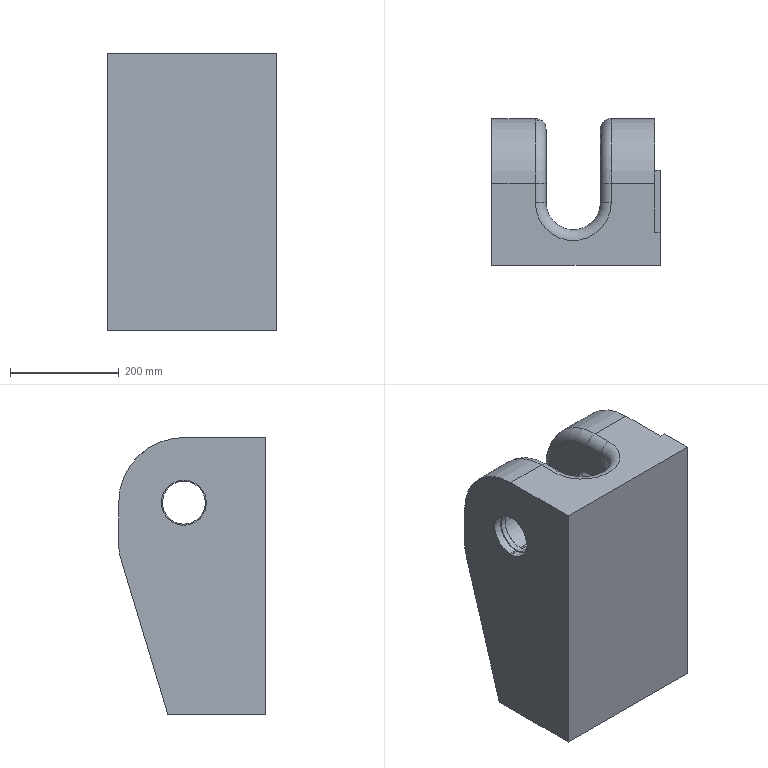Part | NX | features solid 2 | 1 solid | 98 faces | box 310 x 270 x 510 mm | volume 26708228 mm3 | plane 60 | cylinder 30 | torus 7 | spline 1 | commonest cylinder face diameters 83 x12 40 x8 79 x4 100 x2 200 x2 240 x2